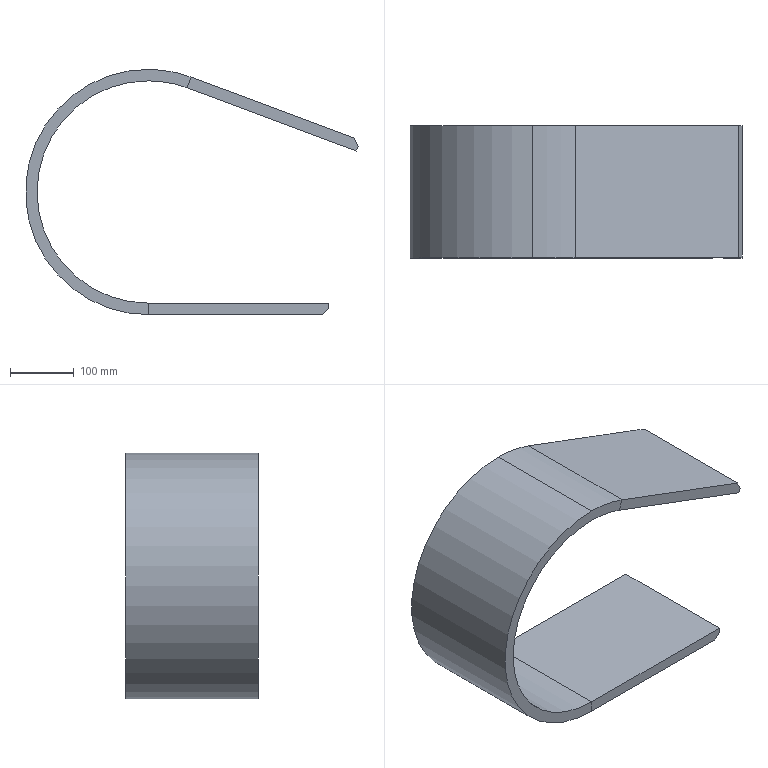Part | SolidWorks | features Chamfer 1, FlatPattern 1, SM3dBend 1, SMBaseFlange 1, SheetMetal 1 | 1 solid | 18 faces | box 521.895 x 207.5 x 385 mm | volume 4494865 mm3 | plane 14 | cylinder 4 | commonest cylinder face diameters 349 x2 385 x2
STEP:
#1=CARTESIAN_POINT('',(925.569,0.,349.));
#2=VERTEX_POINT('',#1);
#3=CARTESIAN_POINT('',(986.68,0.,337.949));
#4=VERTEX_POINT('',#3);
#5=CARTESIAN_POINT('',(925.569,0.,174.5));
#6=DIRECTION('',(0.,1.,0.));
#7=DIRECTION('',(0.,0.,1.));
#8=AXIS2_PLACEMENT_3D('',#5,#6,#7);
#9=CIRCLE('',#8,174.5);
#10=EDGE_CURVE('',#2,#4,#9,.T.);
#11=ORIENTED_EDGE('',*,*,#10,.F.);
#12=CARTESIAN_POINT('',(925.569,207.5,349.));
#13=VERTEX_POINT('',#12);
#14=CARTESIAN_POINT('',(925.569,-571.321,349.));
#15=DIRECTION('',(0.,1.,0.));
#16=VECTOR('',#15,1000.);
#17=LINE('',#14,#16);
#18=EDGE_CURVE('',#2,#13,#17,.T.);
#19=ORIENTED_EDGE('',*,*,#18,.T.);
#20=CARTESIAN_POINT('',(986.68,207.5,337.949));
#21=VERTEX_POINT('',#20);
#22=CARTESIAN_POINT('',(925.569,207.5,174.5));
#23=DIRECTION('',(0.,-1.,0.));
#24=DIRECTION('',(0.,0.,1.));
#25=AXIS2_PLACEMENT_3D('',#22,#23,#24);
#26=CIRCLE('',#25,174.5);
#27=EDGE_CURVE('',#21,#13,#26,.T.);
#28=ORIENTED_EDGE('',*,*,#27,.F.);
#29=CARTESIAN_POINT('',(986.68,207.5,337.949));
#30=DIRECTION('',(0.,-1.,0.));
#31=VECTOR('',#30,1000.);
#32=LINE('',#29,#31);
#33=EDGE_CURVE('',#21,#4,#32,.T.);
#34=ORIENTED_EDGE('',*,*,#33,.T.);
#35=EDGE_LOOP('',(#11,#19,#28,#34));
#36=FACE_OUTER_BOUND('',#35,.T.);
#37=CARTESIAN_POINT('',(925.569,-571.321,174.5));
#38=DIRECTION('',(0.,1.,0.));
#39=DIRECTION('',(0.,0.,1.));
#40=AXIS2_PLACEMENT_3D('',#37,#38,#39);
#41=CYLINDRICAL_SURFACE('',#40,174.5);
#42=ADVANCED_FACE('',(#36),#41,.F.);
#43=CARTESIAN_POINT('',(925.569,0.,-18.));
#44=VERTEX_POINT('',#43);
#45=CARTESIAN_POINT('',(925.569,0.,367.));
#46=VERTEX_POINT('',#45);
#47=CARTESIAN_POINT('',(925.569,0.,174.5));
#48=DIRECTION('',(0.,1.,0.));
#49=DIRECTION('',(0.,0.,-1.));
#50=AXIS2_PLACEMENT_3D('',#47,#48,#49);
#51=CIRCLE('',#50,192.5);
#52=EDGE_CURVE('',#44,#46,#51,.T.);
#53=ORIENTED_EDGE('',*,*,#52,.T.);
#54=CARTESIAN_POINT('',(925.569,207.5,367.));
#55=VERTEX_POINT('',#54);
#56=CARTESIAN_POINT('',(925.569,-571.321,367.));
#57=DIRECTION('',(0.,1.,0.));
#58=VECTOR('',#57,1000.);
#59=LINE('',#56,#58);
#60=EDGE_CURVE('',#46,#55,#59,.T.);
#61=ORIENTED_EDGE('',*,*,#60,.T.);
#62=CARTESIAN_POINT('',(925.569,207.5,-18.));
#63=VERTEX_POINT('',#62);
#64=CARTESIAN_POINT('',(925.569,207.5,174.5));
#65=DIRECTION('',(0.,-1.,0.));
#66=DIRECTION('',(0.,0.,1.));
#67=AXIS2_PLACEMENT_3D('',#64,#65,#66);
#68=CIRCLE('',#67,192.5);
#69=EDGE_CURVE('',#55,#63,#68,.T.);
#70=ORIENTED_EDGE('',*,*,#69,.T.);
#71=CARTESIAN_POINT('',(925.569,207.5,-18.));
#72=DIRECTION('',(0.,-1.,0.));
#73=VECTOR('',#72,1000.);
#74=LINE('',#71,#73);
#75=EDGE_CURVE('',#63,#44,#74,.T.);
#76=ORIENTED_EDGE('',*,*,#75,.T.);
#77=EDGE_LOOP('',(#53,#61,#70,#76));
#78=FACE_OUTER_BOUND('',#77,.T.);
#79=CARTESIAN_POINT('',(925.569,-571.321,174.5));
#80=DIRECTION('',(0.,1.,0.));
#81=DIRECTION('',(0.,0.,1.));
#82=AXIS2_PLACEMENT_3D('',#79,#80,#81);
#83=CYLINDRICAL_SURFACE('',#82,192.5);
#84=ADVANCED_FACE('',(#78),#83,.T.);
#85=CARTESIAN_POINT('',(1252.162,207.5,238.69));
#86=VERTEX_POINT('',#85);
#87=CARTESIAN_POINT('',(1252.162,207.5,238.69));
#88=DIRECTION('',(0.9367,0.,-0.3502));
#89=VECTOR('',#88,1000.);
#90=LINE('',#87,#89);
#91=EDGE_CURVE('',#21,#86,#90,.T.);
#92=ORIENTED_EDGE('',*,*,#91,.F.);
#93=CARTESIAN_POINT('',(992.984,207.5,354.809));
#94=VERTEX_POINT('',#93);
#95=CARTESIAN_POINT('',(992.984,207.5,354.809));
#96=DIRECTION('',(0.3502,0.,0.9367));
#97=VECTOR('',#96,1000.);
#98=LINE('',#95,#97);
#99=EDGE_CURVE('',#21,#94,#98,.T.);
#100=ORIENTED_EDGE('',*,*,#99,.T.);
#101=CARTESIAN_POINT('',(1249.099,207.5,259.052));
#102=VERTEX_POINT('',#101);
#103=CARTESIAN_POINT('',(1258.466,207.5,255.55));
#104=DIRECTION('',(0.9367,0.,-0.3502));
#105=VECTOR('',#104,1000.);
#106=LINE('',#103,#105);
#107=EDGE_CURVE('',#94,#102,#106,.T.);
#108=ORIENTED_EDGE('',*,*,#107,.T.);
#109=CARTESIAN_POINT('',(1254.964,207.5,246.183));
#110=VERTEX_POINT('',#109);
#111=CARTESIAN_POINT('',(1252.031,207.5,252.617));
#112=DIRECTION('',(0.4147,0.,-0.91));
#113=VECTOR('',#112,1000.);
#114=LINE('',#111,#113);
#115=EDGE_CURVE('',#102,#110,#114,.T.);
#116=ORIENTED_EDGE('',*,*,#115,.T.);
#117=CARTESIAN_POINT('',(1258.466,207.5,255.55));
#118=DIRECTION('',(-0.3502,0.,-0.9367));
#119=VECTOR('',#118,1000.);
#120=LINE('',#117,#119);
#121=EDGE_CURVE('',#110,#86,#120,.T.);
#122=ORIENTED_EDGE('',*,*,#121,.T.);
#123=EDGE_LOOP('',(#92,#100,#108,#116,#122));
#124=FACE_OUTER_BOUND('',#123,.T.);
#125=CARTESIAN_POINT('',(1258.466,207.5,255.55));
#126=DIRECTION('',(0.,1.,0.));
#127=DIRECTION('',(0.9367,0.,-0.3502));
#128=AXIS2_PLACEMENT_3D('',#125,#126,#127);
#129=PLANE('',#128);
#130=ADVANCED_FACE('',(#124),#129,.T.);
#131=CARTESIAN_POINT('',(1249.099,0.,259.052));
#132=VERTEX_POINT('',#131);
#133=CARTESIAN_POINT('',(992.984,0.,354.809));
#134=VERTEX_POINT('',#133);
#135=CARTESIAN_POINT('',(1258.466,0.,255.55));
#136=DIRECTION('',(-0.9367,0.,0.3502));
#137=VECTOR('',#136,1000.);
#138=LINE('',#135,#137);
#139=EDGE_CURVE('',#132,#134,#138,.T.);
#140=ORIENTED_EDGE('',*,*,#139,.T.);
#141=CARTESIAN_POINT('',(992.984,0.,354.809));
#142=DIRECTION('',(-0.3502,0.,-0.9367));
#143=VECTOR('',#142,1000.);
#144=LINE('',#141,#143);
#145=EDGE_CURVE('',#134,#4,#144,.T.);
#146=ORIENTED_EDGE('',*,*,#145,.T.);
#147=CARTESIAN_POINT('',(1252.162,0.,238.69));
#148=VERTEX_POINT('',#147);
#149=CARTESIAN_POINT('',(1252.162,0.,238.69));
#150=DIRECTION('',(-0.9367,0.,0.3502));
#151=VECTOR('',#150,1000.);
#152=LINE('',#149,#151);
#153=EDGE_CURVE('',#148,#4,#152,.T.);
#154=ORIENTED_EDGE('',*,*,#153,.F.);
#155=CARTESIAN_POINT('',(1254.964,0.,246.183));
#156=VERTEX_POINT('',#155);
#157=CARTESIAN_POINT('',(1258.466,0.,255.55));
#158=DIRECTION('',(-0.3502,0.,-0.9367));
#159=VECTOR('',#158,1000.);
#160=LINE('',#157,#159);
#161=EDGE_CURVE('',#156,#148,#160,.T.);
#162=ORIENTED_EDGE('',*,*,#161,.F.);
#163=CARTESIAN_POINT('',(1252.031,0.,252.617));
#164=DIRECTION('',(-0.4147,0.,0.91));
#165=VECTOR('',#164,1000.);
#166=LINE('',#163,#165);
#167=EDGE_CURVE('',#156,#132,#166,.T.);
#168=ORIENTED_EDGE('',*,*,#167,.T.);
#169=EDGE_LOOP('',(#140,#146,#154,#162,#168));
#170=FACE_OUTER_BOUND('',#169,.T.);
#171=CARTESIAN_POINT('',(1258.466,0.,255.55));
#172=DIRECTION('',(0.,-1.,0.));
#173=DIRECTION('',(0.3502,0.,0.9367));
#174=AXIS2_PLACEMENT_3D('',#171,#172,#173);
#175=PLANE('',#174);
#176=ADVANCED_FACE('',(#170),#175,.T.);
#177=ORIENTED_EDGE('',*,*,#107,.F.);
#178=CARTESIAN_POINT('',(992.984,207.5,354.809));
#179=DIRECTION('',(0.,-1.,0.));
#180=VECTOR('',#179,1000.);
#181=LINE('',#178,#180);
#182=EDGE_CURVE('',#94,#134,#181,.T.);
#183=ORIENTED_EDGE('',*,*,#182,.T.);
#184=ORIENTED_EDGE('',*,*,#139,.F.);
#185=CARTESIAN_POINT('',(1249.099,207.5,259.052));
#186=DIRECTION('',(0.,1.,0.));
#187=VECTOR('',#186,1000.);
#188=LINE('',#185,#187);
#189=EDGE_CURVE('',#132,#102,#188,.T.);
#190=ORIENTED_EDGE('',*,*,#189,.T.);
#191=EDGE_LOOP('',(#177,#183,#184,#190));
#192=FACE_OUTER_BOUND('',#191,.T.);
#193=CARTESIAN_POINT('',(1258.466,207.5,255.55));
#194=DIRECTION('',(0.3502,0.,0.9367));
#195=DIRECTION('',(0.9367,0.,-0.3502));
#196=AXIS2_PLACEMENT_3D('',#193,#194,#195);
#197=PLANE('',#196);
#198=ADVANCED_FACE('',(#192),#197,.T.);
#199=ORIENTED_EDGE('',*,*,#121,.F.);
#200=CARTESIAN_POINT('',(1254.964,0.,246.183));
#201=DIRECTION('',(0.,-1.,0.));
#202=VECTOR('',#201,1000.);
#203=LINE('',#200,#202);
#204=EDGE_CURVE('',#110,#156,#203,.T.);
#205=ORIENTED_EDGE('',*,*,#204,.T.);
#206=ORIENTED_EDGE('',*,*,#161,.T.);
#207=CARTESIAN_POINT('',(1252.162,0.,238.69));
#208=DIRECTION('',(0.,-1.,0.));
#209=VECTOR('',#208,1000.);
#210=LINE('',#207,#209);
#211=EDGE_CURVE('',#86,#148,#210,.T.);
#212=ORIENTED_EDGE('',*,*,#211,.F.);
#213=EDGE_LOOP('',(#199,#205,#206,#212));
#214=FACE_OUTER_BOUND('',#213,.T.);
#215=CARTESIAN_POINT('',(1258.466,0.,255.55));
#216=DIRECTION('',(0.9367,0.,-0.3502));
#217=DIRECTION('',(-0.3502,0.,-0.9367));
#218=AXIS2_PLACEMENT_3D('',#215,#216,#217);
#219=PLANE('',#218);
#220=ADVANCED_FACE('',(#214),#219,.T.);
#221=ORIENTED_EDGE('',*,*,#33,.F.);
#222=ORIENTED_EDGE('',*,*,#91,.T.);
#223=ORIENTED_EDGE('',*,*,#211,.T.);
#224=ORIENTED_EDGE('',*,*,#153,.T.);
#225=EDGE_LOOP('',(#221,#222,#223,#224));
#226=FACE_OUTER_BOUND('',#225,.T.);
#227=CARTESIAN_POINT('',(1252.162,207.5,238.69));
#228=DIRECTION('',(0.3502,0.,0.9367));
#229=DIRECTION('',(0.9367,0.,-0.3502));
#230=AXIS2_PLACEMENT_3D('',#227,#228,#229);
#231=PLANE('',#230);
#232=ADVANCED_FACE('',(#226),#231,.F.);
#233=ORIENTED_EDGE('',*,*,#115,.F.);
#234=ORIENTED_EDGE('',*,*,#189,.F.);
#235=ORIENTED_EDGE('',*,*,#167,.F.);
#236=ORIENTED_EDGE('',*,*,#204,.F.);
#237=EDGE_LOOP('',(#233,#234,#235,#236));
#238=FACE_OUTER_BOUND('',#237,.T.);
#239=CARTESIAN_POINT('',(1254.964,0.,246.183));
#240=DIRECTION('',(-0.91,0.,-0.4147));
#241=DIRECTION('',(-0.4147,0.,0.91));
#242=AXIS2_PLACEMENT_3D('',#239,#240,#241);
#243=PLANE('',#242);
#244=ADVANCED_FACE('',(#238),#243,.F.);
#245=CARTESIAN_POINT('',(1209.,0.,-8.));
#246=VERTEX_POINT('',#245);
#247=CARTESIAN_POINT('',(1209.,0.,0.));
#248=VERTEX_POINT('',#247);
#249=CARTESIAN_POINT('',(1209.,0.,-18.));
#250=DIRECTION('',(0.,0.,1.));
#251=VECTOR('',#250,1000.);
#252=LINE('',#249,#251);
#253=EDGE_CURVE('',#246,#248,#252,.T.);
#254=ORIENTED_EDGE('',*,*,#253,.F.);
#255=CARTESIAN_POINT('',(1209.,207.5,-8.));
#256=VERTEX_POINT('',#255);
#257=CARTESIAN_POINT('',(1209.,0.,-8.));
#258=DIRECTION('',(0.,1.,0.));
#259=VECTOR('',#258,1000.);
#260=LINE('',#257,#259);
#261=EDGE_CURVE('',#246,#256,#260,.T.);
#262=ORIENTED_EDGE('',*,*,#261,.T.);
#263=CARTESIAN_POINT('',(1209.,207.5,0.));
#264=VERTEX_POINT('',#263);
#265=CARTESIAN_POINT('',(1209.,207.5,-18.));
#266=DIRECTION('',(0.,0.,1.));
#267=VECTOR('',#266,1000.);
#268=LINE('',#265,#267);
#269=EDGE_CURVE('',#256,#264,#268,.T.);
#270=ORIENTED_EDGE('',*,*,#269,.T.);
#271=CARTESIAN_POINT('',(1209.,0.,0.));
#272=DIRECTION('',(0.,1.,0.));
#273=VECTOR('',#272,1000.);
#274=LINE('',#271,#273);
#275=EDGE_CURVE('',#248,#264,#274,.T.);
#276=ORIENTED_EDGE('',*,*,#275,.F.);
#277=EDGE_LOOP('',(#254,#262,#270,#276));
#278=FACE_OUTER_BOUND('',#277,.T.);
#279=CARTESIAN_POINT('',(1209.,0.,-18.));
#280=DIRECTION('',(1.,0.,0.));
#281=DIRECTION('',(0.,0.,-1.));
#282=AXIS2_PLACEMENT_3D('',#279,#280,#281);
#283=PLANE('',#282);
#284=ADVANCED_FACE('',(#278),#283,.T.);
#285=CARTESIAN_POINT('',(1199.,0.,-18.));
#286=VERTEX_POINT('',#285);
#287=CARTESIAN_POINT('',(599.5,0.,-617.5));
#288=DIRECTION('',(0.7071,0.,0.7071));
#289=VECTOR('',#288,1000.);
#290=LINE('',#287,#289);
#291=EDGE_CURVE('',#286,#246,#290,.T.);
#292=ORIENTED_EDGE('',*,*,#291,.F.);
#293=CARTESIAN_POINT('',(1199.,207.5,-18.));
#294=VERTEX_POINT('',#293);
#295=CARTESIAN_POINT('',(1199.,207.5,-18.));
#296=DIRECTION('',(0.,-1.,0.));
#297=VECTOR('',#296,1000.);
#298=LINE('',#295,#297);
#299=EDGE_CURVE('',#294,#286,#298,.T.);
#300=ORIENTED_EDGE('',*,*,#299,.F.);
#301=CARTESIAN_POINT('',(599.5,207.5,-617.5));
#302=DIRECTION('',(-0.7071,0.,-0.7071));
#303=VECTOR('',#302,1000.);
#304=LINE('',#301,#303);
#305=EDGE_CURVE('',#256,#294,#304,.T.);
#306=ORIENTED_EDGE('',*,*,#305,.F.);
#307=ORIENTED_EDGE('',*,*,#261,.F.);
#308=EDGE_LOOP('',(#292,#300,#306,#307));
#309=FACE_OUTER_BOUND('',#308,.T.);
#310=CARTESIAN_POINT('',(1209.,0.,-8.));
#311=DIRECTION('',(-0.7071,0.,0.7071));
#312=DIRECTION('',(0.7071,0.,0.7071));
#313=AXIS2_PLACEMENT_3D('',#310,#311,#312);
#314=PLANE('',#313);
#315=ADVANCED_FACE('',(#309),#314,.F.);
#316=ORIENTED_EDGE('',*,*,#75,.F.);
#317=CARTESIAN_POINT('',(0.,207.5,-18.));
#318=DIRECTION('',(-1.,0.,0.));
#319=VECTOR('',#318,1000.);
#320=LINE('',#317,#319);
#321=EDGE_CURVE('',#294,#63,#320,.T.);
#322=ORIENTED_EDGE('',*,*,#321,.F.);
#323=ORIENTED_EDGE('',*,*,#299,.T.);
#324=CARTESIAN_POINT('',(0.,0.,-18.));
#325=DIRECTION('',(1.,0.,0.));
#326=VECTOR('',#325,1000.);
#327=LINE('',#324,#326);
#328=EDGE_CURVE('',#44,#286,#327,.T.);
#329=ORIENTED_EDGE('',*,*,#328,.F.);
#330=EDGE_LOOP('',(#316,#322,#323,#329));
#331=FACE_OUTER_BOUND('',#330,.T.);
#332=CARTESIAN_POINT('',(0.,207.5,-18.));
#333=DIRECTION('',(0.,0.,-1.));
#334=DIRECTION('',(-1.,0.,0.));
#335=AXIS2_PLACEMENT_3D('',#332,#333,#334);
#336=PLANE('',#335);
#337=ADVANCED_FACE('',(#331),#336,.T.);
#338=CARTESIAN_POINT('',(925.569,207.5,0.));
#339=VERTEX_POINT('',#338);
#340=CARTESIAN_POINT('',(925.569,207.5,-18.));
#341=DIRECTION('',(0.,0.,-1.));
#342=VECTOR('',#341,1000.);
#343=LINE('',#340,#342);
#344=EDGE_CURVE('',#339,#63,#343,.T.);
#345=ORIENTED_EDGE('',*,*,#344,.F.);
#346=CARTESIAN_POINT('',(0.,207.5,0.));
#347=DIRECTION('',(-1.,0.,0.));
#348=VECTOR('',#347,1000.);
#349=LINE('',#346,#348);
#350=EDGE_CURVE('',#264,#339,#349,.T.);
#351=ORIENTED_EDGE('',*,*,#350,.F.);
#352=ORIENTED_EDGE('',*,*,#269,.F.);
#353=ORIENTED_EDGE('',*,*,#305,.T.);
#354=ORIENTED_EDGE('',*,*,#321,.T.);
#355=EDGE_LOOP('',(#345,#351,#352,#353,#354));
#356=FACE_OUTER_BOUND('',#355,.T.);
#357=CARTESIAN_POINT('',(0.,207.5,-18.));
#358=DIRECTION('',(0.,1.,0.));
#359=DIRECTION('',(-1.,0.,0.));
#360=AXIS2_PLACEMENT_3D('',#357,#358,#359);
#361=PLANE('',#360);
#362=ADVANCED_FACE('',(#356),#361,.T.);
#363=ORIENTED_EDGE('',*,*,#350,.T.);
#364=CARTESIAN_POINT('',(925.569,0.,0.));
#365=VERTEX_POINT('',#364);
#366=CARTESIAN_POINT('',(925.569,207.5,0.));
#367=DIRECTION('',(0.,-1.,0.));
#368=VECTOR('',#367,1000.);
#369=LINE('',#366,#368);
#370=EDGE_CURVE('',#339,#365,#369,.T.);
#371=ORIENTED_EDGE('',*,*,#370,.T.);
#372=CARTESIAN_POINT('',(0.,0.,0.));
#373=DIRECTION('',(1.,0.,0.));
#374=VECTOR('',#373,1000.);
#375=LINE('',#372,#374);
#376=EDGE_CURVE('',#365,#248,#375,.T.);
#377=ORIENTED_EDGE('',*,*,#376,.T.);
#378=ORIENTED_EDGE('',*,*,#275,.T.);
#379=EDGE_LOOP('',(#363,#371,#377,#378));
#380=FACE_OUTER_BOUND('',#379,.T.);
#381=CARTESIAN_POINT('',(0.,207.5,0.));
#382=DIRECTION('',(0.,0.,-1.));
#383=DIRECTION('',(-1.,0.,0.));
#384=AXIS2_PLACEMENT_3D('',#381,#382,#383);
#385=PLANE('',#384);
#386=ADVANCED_FACE('',(#380),#385,.F.);
#387=CARTESIAN_POINT('',(925.569,0.,-18.));
#388=DIRECTION('',(0.,0.,1.));
#389=VECTOR('',#388,1000.);
#390=LINE('',#387,#389);
#391=EDGE_CURVE('',#44,#365,#390,.T.);
#392=ORIENTED_EDGE('',*,*,#391,.F.);
#393=ORIENTED_EDGE('',*,*,#328,.T.);
#394=ORIENTED_EDGE('',*,*,#291,.T.);
#395=ORIENTED_EDGE('',*,*,#253,.T.);
#396=ORIENTED_EDGE('',*,*,#376,.F.);
#397=EDGE_LOOP('',(#392,#393,#394,#395,#396));
#398=FACE_OUTER_BOUND('',#397,.T.);
#399=CARTESIAN_POINT('',(0.,0.,-18.));
#400=DIRECTION('',(0.,-1.,0.));
#401=DIRECTION('',(0.,0.,-1.));
#402=AXIS2_PLACEMENT_3D('',#399,#400,#401);
#403=PLANE('',#402);
#404=ADVANCED_FACE('',(#398),#403,.T.);
#405=ORIENTED_EDGE('',*,*,#99,.F.);
#406=ORIENTED_EDGE('',*,*,#27,.T.);
#407=CARTESIAN_POINT('',(925.569,207.5,174.5));
#408=DIRECTION('',(0.,-1.,0.));
#409=DIRECTION('',(0.,0.,1.));
#410=AXIS2_PLACEMENT_3D('',#407,#408,#409);
#411=CIRCLE('',#410,174.5);
#412=EDGE_CURVE('',#13,#339,#411,.T.);
#413=ORIENTED_EDGE('',*,*,#412,.T.);
#414=ORIENTED_EDGE('',*,*,#344,.T.);
#415=ORIENTED_EDGE('',*,*,#69,.F.);
#416=CARTESIAN_POINT('',(925.569,207.5,174.5));
#417=DIRECTION('',(0.,-1.,0.));
#418=DIRECTION('',(0.,0.,1.));
#419=AXIS2_PLACEMENT_3D('',#416,#417,#418);
#420=CIRCLE('',#419,192.5);
#421=EDGE_CURVE('',#94,#55,#420,.T.);
#422=ORIENTED_EDGE('',*,*,#421,.F.);
#423=EDGE_LOOP('',(#405,#406,#413,#414,#415,#422));
#424=FACE_OUTER_BOUND('',#423,.T.);
#425=CARTESIAN_POINT('',(925.569,207.5,174.5));
#426=DIRECTION('',(0.,1.,0.));
#427=DIRECTION('',(0.,0.,1.));
#428=AXIS2_PLACEMENT_3D('',#425,#426,#427);
#429=PLANE('',#428);
#430=ADVANCED_FACE('',(#424),#429,.T.);
#431=ORIENTED_EDGE('',*,*,#60,.F.);
#432=CARTESIAN_POINT('',(925.569,0.,174.5));
#433=DIRECTION('',(0.,1.,0.));
#434=DIRECTION('',(0.,0.,-1.));
#435=AXIS2_PLACEMENT_3D('',#432,#433,#434);
#436=CIRCLE('',#435,192.5);
#437=EDGE_CURVE('',#46,#134,#436,.T.);
#438=ORIENTED_EDGE('',*,*,#437,.T.);
#439=ORIENTED_EDGE('',*,*,#182,.F.);
#440=ORIENTED_EDGE('',*,*,#421,.T.);
#441=EDGE_LOOP('',(#431,#438,#439,#440));
#442=FACE_OUTER_BOUND('',#441,.T.);
#443=CARTESIAN_POINT('',(925.569,-571.321,174.5));
#444=DIRECTION('',(0.,1.,0.));
#445=DIRECTION('',(0.,0.,1.));
#446=AXIS2_PLACEMENT_3D('',#443,#444,#445);
#447=CYLINDRICAL_SURFACE('',#446,192.5);
#448=ADVANCED_FACE('',(#442),#447,.T.);
#449=CARTESIAN_POINT('',(925.569,0.,174.5));
#450=DIRECTION('',(0.,1.,0.));
#451=DIRECTION('',(0.,0.,1.));
#452=AXIS2_PLACEMENT_3D('',#449,#450,#451);
#453=CIRCLE('',#452,174.5);
#454=EDGE_CURVE('',#365,#2,#453,.T.);
#455=ORIENTED_EDGE('',*,*,#454,.T.);
#456=ORIENTED_EDGE('',*,*,#10,.T.);
#457=ORIENTED_EDGE('',*,*,#145,.F.);
#458=ORIENTED_EDGE('',*,*,#437,.F.);
#459=ORIENTED_EDGE('',*,*,#52,.F.);
#460=ORIENTED_EDGE('',*,*,#391,.T.);
#461=EDGE_LOOP('',(#455,#456,#457,#458,#459,#460));
#462=FACE_OUTER_BOUND('',#461,.T.);
#463=CARTESIAN_POINT('',(925.569,0.,174.5));
#464=DIRECTION('',(0.,-1.,0.));
#465=DIRECTION('',(0.,0.,-1.));
#466=AXIS2_PLACEMENT_3D('',#463,#464,#465);
#467=PLANE('',#466);
#468=ADVANCED_FACE('',(#462),#467,.T.);
#469=ORIENTED_EDGE('',*,*,#18,.F.);
#470=ORIENTED_EDGE('',*,*,#454,.F.);
#471=ORIENTED_EDGE('',*,*,#370,.F.);
#472=ORIENTED_EDGE('',*,*,#412,.F.);
#473=EDGE_LOOP('',(#469,#470,#471,#472));
#474=FACE_OUTER_BOUND('',#473,.T.);
#475=CARTESIAN_POINT('',(925.569,-571.321,174.5));
#476=DIRECTION('',(0.,1.,0.));
#477=DIRECTION('',(0.,0.,1.));
#478=AXIS2_PLACEMENT_3D('',#475,#476,#477);
#479=CYLINDRICAL_SURFACE('',#478,174.5);
#480=ADVANCED_FACE('',(#474),#479,.F.);
#481=CLOSED_SHELL('',(#42,#84,#130,#176,#198,#220,#232,#244,#284,#315,#337,#362,#386,#404,#430,#448,#468,#480));
#482=MANIFOLD_SOLID_BREP('',#481);
#483=CARTESIAN_POINT('',(0.,0.,0.));
#484=DIRECTION('',(0.,0.,1.));
#485=DIRECTION('',(1.,0.,0.));
#486=AXIS2_PLACEMENT_3D('',#483,#484,#485);
#487=(LENGTH_UNIT()NAMED_UNIT(*)SI_UNIT(.MILLI.,.METRE.));
#488=UNCERTAINTY_MEASURE_WITH_UNIT(LENGTH_MEASURE(0.00001),#487,'','');
#489=(NAMED_UNIT(*)PLANE_ANGLE_UNIT()SI_UNIT($,.RADIAN.));
#490=(NAMED_UNIT(*)SI_UNIT($,.STERADIAN.)SOLID_ANGLE_UNIT());
#491=(GEOMETRIC_REPRESENTATION_CONTEXT(3)GLOBAL_UNCERTAINTY_ASSIGNED_CONTEXT((#488))GLOBAL_UNIT_ASSIGNED_CONTEXT((#487,#489,#490))REPRESENTATION_CONTEXT('',''));
#492=ADVANCED_BREP_SHAPE_REPRESENTATION('',(#482,#486),#491);